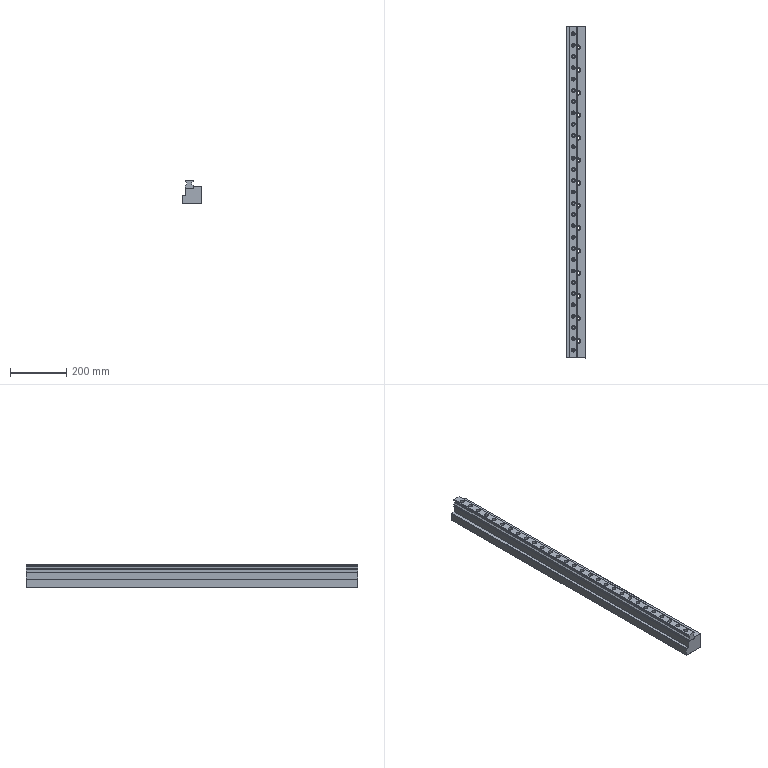Part | SolidWorks | 2 solids | 423 faces | box 70 x 1176 x 83 mm | volume 4869056 mm3 | cylinder 260 | plane 160 | cone 3 | commonest cylinder face diameters 6.5 x58 9 x58 14 x58 2 x30 11 x28 17.5 x28